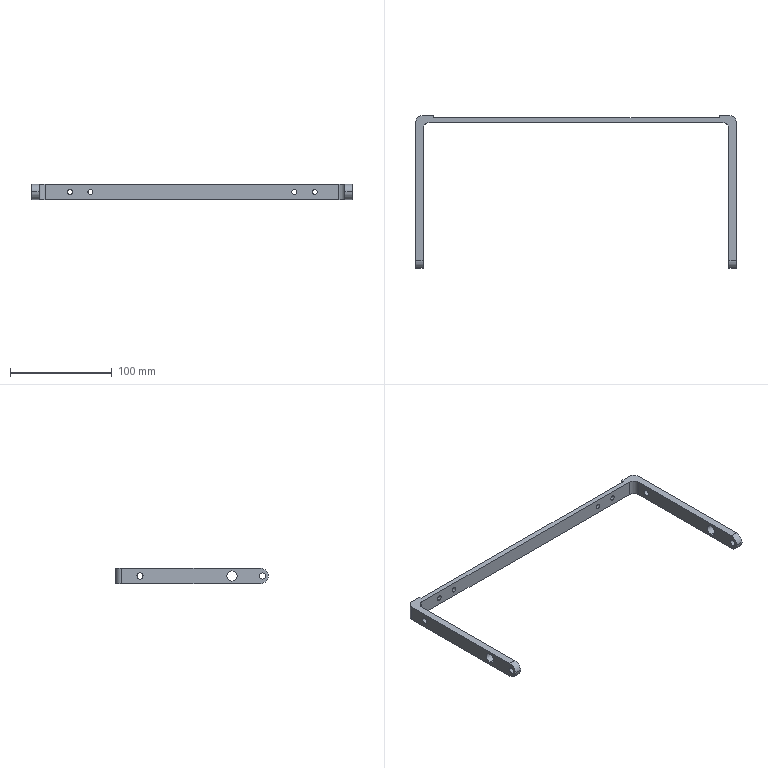Part | SolidWorks | features ICE 3, Fillet 2, Cut 1, Extrusion 1 | 1 solid | 40 faces | box 314 x 149.984 x 15 mm | volume 51932 mm3 | cylinder 28 | plane 12 | commonest cylinder face diameters 5 x8 6 x8 10 x4 12 x4 16 x4
STEP:
#1=CARTESIAN_POINT('',(157.,30.,2.5));
#2=VERTEX_POINT('',#1);
#3=CARTESIAN_POINT('',(157.,30.,12.5));
#4=VERTEX_POINT('',#3);
#5=CARTESIAN_POINT('',(157.,30.,7.5));
#6=DIRECTION('',(-1.,0.,0.));
#7=DIRECTION('',(0.,0.,1.));
#8=AXIS2_PLACEMENT_3D('',#5,#6,#7);
#9=CIRCLE('',#8,5.);
#10=EDGE_CURVE('',#2,#4,#9,.T.);
#11=ORIENTED_EDGE('',*,*,#10,.F.);
#12=CARTESIAN_POINT('',(150.,30.,2.5));
#13=VERTEX_POINT('',#12);
#14=CARTESIAN_POINT('',(157.,30.,2.5));
#15=DIRECTION('',(-1.,0.,0.));
#16=VECTOR('',#15,1000.);
#17=LINE('',#14,#16);
#18=EDGE_CURVE('',#2,#13,#17,.T.);
#19=ORIENTED_EDGE('',*,*,#18,.T.);
#20=CARTESIAN_POINT('',(150.,30.,12.5));
#21=VERTEX_POINT('',#20);
#22=CARTESIAN_POINT('',(150.,30.,7.5));
#23=DIRECTION('',(1.,0.,0.));
#24=DIRECTION('',(0.,1.,0.));
#25=AXIS2_PLACEMENT_3D('',#22,#23,#24);
#26=CIRCLE('',#25,5.);
#27=EDGE_CURVE('',#21,#13,#26,.T.);
#28=ORIENTED_EDGE('',*,*,#27,.F.);
#29=CARTESIAN_POINT('',(157.,30.,12.5));
#30=DIRECTION('',(-1.,0.,0.));
#31=VECTOR('',#30,1000.);
#32=LINE('',#29,#31);
#33=EDGE_CURVE('',#4,#21,#32,.T.);
#34=ORIENTED_EDGE('',*,*,#33,.F.);
#35=EDGE_LOOP('',(#11,#19,#28,#34));
#36=FACE_OUTER_BOUND('',#35,.T.);
#37=CARTESIAN_POINT('',(157.,30.,7.5));
#38=DIRECTION('',(-1.,0.,0.));
#39=DIRECTION('',(0.,0.,1.));
#40=AXIS2_PLACEMENT_3D('',#37,#38,#39);
#41=CYLINDRICAL_SURFACE('',#40,5.);
#42=ADVANCED_FACE('',(#36),#41,.F.);
#43=CARTESIAN_POINT('',(-150.,30.,2.5));
#44=VERTEX_POINT('',#43);
#45=CARTESIAN_POINT('',(-150.,30.,12.5));
#46=VERTEX_POINT('',#45);
#47=CARTESIAN_POINT('',(-150.,30.,7.5));
#48=DIRECTION('',(-1.,0.,0.));
#49=DIRECTION('',(0.,-1.,0.));
#50=AXIS2_PLACEMENT_3D('',#47,#48,#49);
#51=CIRCLE('',#50,5.);
#52=EDGE_CURVE('',#44,#46,#51,.T.);
#53=ORIENTED_EDGE('',*,*,#52,.F.);
#54=CARTESIAN_POINT('',(-157.,30.,2.5));
#55=VERTEX_POINT('',#54);
#56=CARTESIAN_POINT('',(157.,30.,2.5));
#57=DIRECTION('',(-1.,0.,0.));
#58=VECTOR('',#57,1000.);
#59=LINE('',#56,#58);
#60=EDGE_CURVE('',#44,#55,#59,.T.);
#61=ORIENTED_EDGE('',*,*,#60,.T.);
#62=CARTESIAN_POINT('',(-157.,30.,12.5));
#63=VERTEX_POINT('',#62);
#64=CARTESIAN_POINT('',(-157.,30.,7.5));
#65=DIRECTION('',(-1.,0.,0.));
#66=DIRECTION('',(0.,0.,1.));
#67=AXIS2_PLACEMENT_3D('',#64,#65,#66);
#68=CIRCLE('',#67,5.);
#69=EDGE_CURVE('',#55,#63,#68,.T.);
#70=ORIENTED_EDGE('',*,*,#69,.T.);
#71=CARTESIAN_POINT('',(157.,30.,12.5));
#72=DIRECTION('',(-1.,0.,0.));
#73=VECTOR('',#72,1000.);
#74=LINE('',#71,#73);
#75=EDGE_CURVE('',#46,#63,#74,.T.);
#76=ORIENTED_EDGE('',*,*,#75,.F.);
#77=EDGE_LOOP('',(#53,#61,#70,#76));
#78=FACE_OUTER_BOUND('',#77,.T.);
#79=CARTESIAN_POINT('',(157.,30.,7.5));
#80=DIRECTION('',(-1.,0.,0.));
#81=DIRECTION('',(0.,0.,1.));
#82=AXIS2_PLACEMENT_3D('',#79,#80,#81);
#83=CYLINDRICAL_SURFACE('',#82,5.);
#84=ADVANCED_FACE('',(#78),#83,.F.);
#85=CARTESIAN_POINT('',(120.39,137.174,5.));
#86=VERTEX_POINT('',#85);
#87=CARTESIAN_POINT('',(120.39,137.174,10.));
#88=VERTEX_POINT('',#87);
#89=CARTESIAN_POINT('',(120.39,137.174,7.5));
#90=DIRECTION('',(0.,1.,0.));
#91=DIRECTION('',(-1.,0.,0.));
#92=AXIS2_PLACEMENT_3D('',#89,#90,#91);
#93=CIRCLE('',#92,2.5);
#94=EDGE_CURVE('',#86,#88,#93,.T.);
#95=ORIENTED_EDGE('',*,*,#94,.F.);
#96=CARTESIAN_POINT('',(120.39,142.174,5.));
#97=VERTEX_POINT('',#96);
#98=CARTESIAN_POINT('',(120.39,-137.826,5.));
#99=DIRECTION('',(0.,1.,0.));
#100=VECTOR('',#99,1000.);
#101=LINE('',#98,#100);
#102=EDGE_CURVE('',#86,#97,#101,.T.);
#103=ORIENTED_EDGE('',*,*,#102,.T.);
#104=CARTESIAN_POINT('',(120.39,142.174,10.));
#105=VERTEX_POINT('',#104);
#106=CARTESIAN_POINT('',(120.39,142.174,7.5));
#107=DIRECTION('',(0.,1.,0.));
#108=DIRECTION('',(0.,0.,1.));
#109=AXIS2_PLACEMENT_3D('',#106,#107,#108);
#110=CIRCLE('',#109,2.5);
#111=EDGE_CURVE('',#97,#105,#110,.T.);
#112=ORIENTED_EDGE('',*,*,#111,.T.);
#113=CARTESIAN_POINT('',(120.39,-137.826,10.));
#114=DIRECTION('',(0.,1.,0.));
#115=VECTOR('',#114,1000.);
#116=LINE('',#113,#115);
#117=EDGE_CURVE('',#88,#105,#116,.T.);
#118=ORIENTED_EDGE('',*,*,#117,.F.);
#119=EDGE_LOOP('',(#95,#103,#112,#118));
#120=FACE_OUTER_BOUND('',#119,.T.);
#121=CARTESIAN_POINT('',(120.39,-137.826,7.5));
#122=DIRECTION('',(0.,1.,0.));
#123=DIRECTION('',(0.,0.,1.));
#124=AXIS2_PLACEMENT_3D('',#121,#122,#123);
#125=CYLINDRICAL_SURFACE('',#124,2.5);
#126=ADVANCED_FACE('',(#120),#125,.F.);
#127=CARTESIAN_POINT('',(-99.61,137.174,5.));
#128=VERTEX_POINT('',#127);
#129=CARTESIAN_POINT('',(-99.61,137.174,10.));
#130=VERTEX_POINT('',#129);
#131=CARTESIAN_POINT('',(-99.61,137.174,7.5));
#132=DIRECTION('',(0.,1.,0.));
#133=DIRECTION('',(-1.,0.,0.));
#134=AXIS2_PLACEMENT_3D('',#131,#132,#133);
#135=CIRCLE('',#134,2.5);
#136=EDGE_CURVE('',#128,#130,#135,.T.);
#137=ORIENTED_EDGE('',*,*,#136,.F.);
#138=CARTESIAN_POINT('',(-99.61,142.174,5.));
#139=VERTEX_POINT('',#138);
#140=CARTESIAN_POINT('',(-99.61,-137.826,5.));
#141=DIRECTION('',(0.,1.,0.));
#142=VECTOR('',#141,1000.);
#143=LINE('',#140,#142);
#144=EDGE_CURVE('',#128,#139,#143,.T.);
#145=ORIENTED_EDGE('',*,*,#144,.T.);
#146=CARTESIAN_POINT('',(-99.61,142.174,10.));
#147=VERTEX_POINT('',#146);
#148=CARTESIAN_POINT('',(-99.61,142.174,7.5));
#149=DIRECTION('',(0.,1.,0.));
#150=DIRECTION('',(0.,0.,1.));
#151=AXIS2_PLACEMENT_3D('',#148,#149,#150);
#152=CIRCLE('',#151,2.5);
#153=EDGE_CURVE('',#139,#147,#152,.T.);
#154=ORIENTED_EDGE('',*,*,#153,.T.);
#155=CARTESIAN_POINT('',(-99.61,-137.826,10.));
#156=DIRECTION('',(0.,1.,0.));
#157=VECTOR('',#156,1000.);
#158=LINE('',#155,#157);
#159=EDGE_CURVE('',#130,#147,#158,.T.);
#160=ORIENTED_EDGE('',*,*,#159,.F.);
#161=EDGE_LOOP('',(#137,#145,#154,#160));
#162=FACE_OUTER_BOUND('',#161,.T.);
#163=CARTESIAN_POINT('',(-99.61,-137.826,7.5));
#164=DIRECTION('',(0.,1.,0.));
#165=DIRECTION('',(0.,0.,1.));
#166=AXIS2_PLACEMENT_3D('',#163,#164,#165);
#167=CYLINDRICAL_SURFACE('',#166,2.5);
#168=ADVANCED_FACE('',(#162),#167,.F.);
#169=CARTESIAN_POINT('',(-119.61,137.174,5.));
#170=VERTEX_POINT('',#169);
#171=CARTESIAN_POINT('',(-119.61,137.174,10.));
#172=VERTEX_POINT('',#171);
#173=CARTESIAN_POINT('',(-119.61,137.174,7.5));
#174=DIRECTION('',(0.,1.,0.));
#175=DIRECTION('',(-1.,0.,0.));
#176=AXIS2_PLACEMENT_3D('',#173,#174,#175);
#177=CIRCLE('',#176,2.5);
#178=EDGE_CURVE('',#170,#172,#177,.T.);
#179=ORIENTED_EDGE('',*,*,#178,.F.);
#180=CARTESIAN_POINT('',(-119.61,142.174,5.));
#181=VERTEX_POINT('',#180);
#182=CARTESIAN_POINT('',(-119.61,-137.826,5.));
#183=DIRECTION('',(0.,1.,0.));
#184=VECTOR('',#183,1000.);
#185=LINE('',#182,#184);
#186=EDGE_CURVE('',#170,#181,#185,.T.);
#187=ORIENTED_EDGE('',*,*,#186,.T.);
#188=CARTESIAN_POINT('',(-119.61,142.174,10.));
#189=VERTEX_POINT('',#188);
#190=CARTESIAN_POINT('',(-119.61,142.174,7.5));
#191=DIRECTION('',(0.,1.,0.));
#192=DIRECTION('',(0.,0.,1.));
#193=AXIS2_PLACEMENT_3D('',#190,#191,#192);
#194=CIRCLE('',#193,2.5);
#195=EDGE_CURVE('',#181,#189,#194,.T.);
#196=ORIENTED_EDGE('',*,*,#195,.T.);
#197=CARTESIAN_POINT('',(-119.61,-137.826,10.));
#198=DIRECTION('',(0.,1.,0.));
#199=VECTOR('',#198,1000.);
#200=LINE('',#197,#199);
#201=EDGE_CURVE('',#172,#189,#200,.T.);
#202=ORIENTED_EDGE('',*,*,#201,.F.);
#203=EDGE_LOOP('',(#179,#187,#196,#202));
#204=FACE_OUTER_BOUND('',#203,.T.);
#205=CARTESIAN_POINT('',(-119.61,-137.826,7.5));
#206=DIRECTION('',(0.,1.,0.));
#207=DIRECTION('',(0.,0.,1.));
#208=AXIS2_PLACEMENT_3D('',#205,#206,#207);
#209=CYLINDRICAL_SURFACE('',#208,2.5);
#210=ADVANCED_FACE('',(#204),#209,.F.);
#211=CARTESIAN_POINT('',(100.39,137.174,5.));
#212=VERTEX_POINT('',#211);
#213=CARTESIAN_POINT('',(100.39,137.174,10.));
#214=VERTEX_POINT('',#213);
#215=CARTESIAN_POINT('',(100.39,137.174,7.5));
#216=DIRECTION('',(0.,1.,0.));
#217=DIRECTION('',(-1.,0.,0.));
#218=AXIS2_PLACEMENT_3D('',#215,#216,#217);
#219=CIRCLE('',#218,2.5);
#220=EDGE_CURVE('',#212,#214,#219,.T.);
#221=ORIENTED_EDGE('',*,*,#220,.F.);
#222=CARTESIAN_POINT('',(100.39,142.174,5.));
#223=VERTEX_POINT('',#222);
#224=CARTESIAN_POINT('',(100.39,-137.826,5.));
#225=DIRECTION('',(0.,1.,0.));
#226=VECTOR('',#225,1000.);
#227=LINE('',#224,#226);
#228=EDGE_CURVE('',#212,#223,#227,.T.);
#229=ORIENTED_EDGE('',*,*,#228,.T.);
#230=CARTESIAN_POINT('',(100.39,142.174,10.));
#231=VERTEX_POINT('',#230);
#232=CARTESIAN_POINT('',(100.39,142.174,7.5));
#233=DIRECTION('',(0.,1.,0.));
#234=DIRECTION('',(0.,0.,1.));
#235=AXIS2_PLACEMENT_3D('',#232,#233,#234);
#236=CIRCLE('',#235,2.5);
#237=EDGE_CURVE('',#223,#231,#236,.T.);
#238=ORIENTED_EDGE('',*,*,#237,.T.);
#239=CARTESIAN_POINT('',(100.39,-137.826,10.));
#240=DIRECTION('',(0.,1.,0.));
#241=VECTOR('',#240,1000.);
#242=LINE('',#239,#241);
#243=EDGE_CURVE('',#214,#231,#242,.T.);
#244=ORIENTED_EDGE('',*,*,#243,.F.);
#245=EDGE_LOOP('',(#221,#229,#238,#244));
#246=FACE_OUTER_BOUND('',#245,.T.);
#247=CARTESIAN_POINT('',(100.39,-137.826,7.5));
#248=DIRECTION('',(0.,1.,0.));
#249=DIRECTION('',(0.,0.,1.));
#250=AXIS2_PLACEMENT_3D('',#247,#248,#249);
#251=CYLINDRICAL_SURFACE('',#250,2.5);
#252=ADVANCED_FACE('',(#246),#251,.F.);
#253=CARTESIAN_POINT('',(150.,-2.826,7.5));
#254=VERTEX_POINT('',#253);
#255=CARTESIAN_POINT('',(150.,3.174,7.5));
#256=VERTEX_POINT('',#255);
#257=CARTESIAN_POINT('',(150.,0.1739,7.5));
#258=DIRECTION('',(1.,0.,0.));
#259=DIRECTION('',(0.,1.,0.));
#260=AXIS2_PLACEMENT_3D('',#257,#258,#259);
#261=CIRCLE('',#260,3.);
#262=EDGE_CURVE('',#254,#256,#261,.T.);
#263=ORIENTED_EDGE('',*,*,#262,.F.);
#264=CARTESIAN_POINT('',(157.,-2.826,7.5));
#265=VERTEX_POINT('',#264);
#266=CARTESIAN_POINT('',(-449.,-2.826,7.5));
#267=DIRECTION('',(1.,0.,0.));
#268=VECTOR('',#267,1000.);
#269=LINE('',#266,#268);
#270=EDGE_CURVE('',#254,#265,#269,.T.);
#271=ORIENTED_EDGE('',*,*,#270,.T.);
#272=CARTESIAN_POINT('',(157.,3.174,7.5));
#273=VERTEX_POINT('',#272);
#274=CARTESIAN_POINT('',(157.,0.1739,7.5));
#275=DIRECTION('',(1.,0.,0.));
#276=DIRECTION('',(0.,1.,0.));
#277=AXIS2_PLACEMENT_3D('',#274,#275,#276);
#278=CIRCLE('',#277,3.);
#279=EDGE_CURVE('',#265,#273,#278,.T.);
#280=ORIENTED_EDGE('',*,*,#279,.T.);
#281=CARTESIAN_POINT('',(-449.,3.174,7.5));
#282=DIRECTION('',(1.,0.,0.));
#283=VECTOR('',#282,1000.);
#284=LINE('',#281,#283);
#285=EDGE_CURVE('',#256,#273,#284,.T.);
#286=ORIENTED_EDGE('',*,*,#285,.F.);
#287=EDGE_LOOP('',(#263,#271,#280,#286));
#288=FACE_OUTER_BOUND('',#287,.T.);
#289=CARTESIAN_POINT('',(-449.,0.1739,7.5));
#290=DIRECTION('',(1.,0.,0.));
#291=DIRECTION('',(0.,1.,0.));
#292=AXIS2_PLACEMENT_3D('',#289,#290,#291);
#293=CYLINDRICAL_SURFACE('',#292,3.);
#294=ADVANCED_FACE('',(#288),#293,.F.);
#295=CARTESIAN_POINT('',(150.,117.174,7.5));
#296=VERTEX_POINT('',#295);
#297=CARTESIAN_POINT('',(150.,123.174,7.5));
#298=VERTEX_POINT('',#297);
#299=CARTESIAN_POINT('',(150.,120.174,7.5));
#300=DIRECTION('',(1.,0.,0.));
#301=DIRECTION('',(0.,1.,0.));
#302=AXIS2_PLACEMENT_3D('',#299,#300,#301);
#303=CIRCLE('',#302,3.);
#304=EDGE_CURVE('',#296,#298,#303,.T.);
#305=ORIENTED_EDGE('',*,*,#304,.F.);
#306=CARTESIAN_POINT('',(157.,117.174,7.5));
#307=VERTEX_POINT('',#306);
#308=CARTESIAN_POINT('',(-449.,117.174,7.5));
#309=DIRECTION('',(1.,0.,0.));
#310=VECTOR('',#309,1000.);
#311=LINE('',#308,#310);
#312=EDGE_CURVE('',#296,#307,#311,.T.);
#313=ORIENTED_EDGE('',*,*,#312,.T.);
#314=CARTESIAN_POINT('',(157.,123.174,7.5));
#315=VERTEX_POINT('',#314);
#316=CARTESIAN_POINT('',(157.,120.174,7.5));
#317=DIRECTION('',(1.,0.,0.));
#318=DIRECTION('',(0.,1.,0.));
#319=AXIS2_PLACEMENT_3D('',#316,#317,#318);
#320=CIRCLE('',#319,3.);
#321=EDGE_CURVE('',#307,#315,#320,.T.);
#322=ORIENTED_EDGE('',*,*,#321,.T.);
#323=CARTESIAN_POINT('',(-449.,123.174,7.5));
#324=DIRECTION('',(1.,0.,0.));
#325=VECTOR('',#324,1000.);
#326=LINE('',#323,#325);
#327=EDGE_CURVE('',#298,#315,#326,.T.);
#328=ORIENTED_EDGE('',*,*,#327,.F.);
#329=EDGE_LOOP('',(#305,#313,#322,#328));
#330=FACE_OUTER_BOUND('',#329,.T.);
#331=CARTESIAN_POINT('',(-449.,120.174,7.5));
#332=DIRECTION('',(1.,0.,0.));
#333=DIRECTION('',(0.,1.,0.));
#334=AXIS2_PLACEMENT_3D('',#331,#332,#333);
#335=CYLINDRICAL_SURFACE('',#334,3.);
#336=ADVANCED_FACE('',(#330),#335,.F.);
#337=CARTESIAN_POINT('',(-157.,-2.826,7.5));
#338=VERTEX_POINT('',#337);
#339=CARTESIAN_POINT('',(-157.,3.174,7.5));
#340=VERTEX_POINT('',#339);
#341=CARTESIAN_POINT('',(-157.,0.1739,7.5));
#342=DIRECTION('',(1.,0.,0.));
#343=DIRECTION('',(0.,0.,-1.));
#344=AXIS2_PLACEMENT_3D('',#341,#342,#343);
#345=CIRCLE('',#344,3.);
#346=EDGE_CURVE('',#338,#340,#345,.T.);
#347=ORIENTED_EDGE('',*,*,#346,.F.);
#348=CARTESIAN_POINT('',(-150.,-2.826,7.5));
#349=VERTEX_POINT('',#348);
#350=CARTESIAN_POINT('',(-449.,-2.826,7.5));
#351=DIRECTION('',(1.,0.,0.));
#352=VECTOR('',#351,1000.);
#353=LINE('',#350,#352);
#354=EDGE_CURVE('',#338,#349,#353,.T.);
#355=ORIENTED_EDGE('',*,*,#354,.T.);
#356=CARTESIAN_POINT('',(-150.,3.174,7.5));
#357=VERTEX_POINT('',#356);
#358=CARTESIAN_POINT('',(-150.,0.1739,7.5));
#359=DIRECTION('',(-1.,0.,0.));
#360=DIRECTION('',(0.,-1.,0.));
#361=AXIS2_PLACEMENT_3D('',#358,#359,#360);
#362=CIRCLE('',#361,3.);
#363=EDGE_CURVE('',#357,#349,#362,.T.);
#364=ORIENTED_EDGE('',*,*,#363,.F.);
#365=CARTESIAN_POINT('',(-449.,3.174,7.5));
#366=DIRECTION('',(1.,0.,0.));
#367=VECTOR('',#366,1000.);
#368=LINE('',#365,#367);
#369=EDGE_CURVE('',#340,#357,#368,.T.);
#370=ORIENTED_EDGE('',*,*,#369,.F.);
#371=EDGE_LOOP('',(#347,#355,#364,#370));
#372=FACE_OUTER_BOUND('',#371,.T.);
#373=CARTESIAN_POINT('',(-449.,0.1739,7.5));
#374=DIRECTION('',(1.,0.,0.));
#375=DIRECTION('',(0.,1.,0.));
#376=AXIS2_PLACEMENT_3D('',#373,#374,#375);
#377=CYLINDRICAL_SURFACE('',#376,3.);
#378=ADVANCED_FACE('',(#372),#377,.F.);
#379=CARTESIAN_POINT('',(-157.,117.174,7.5));
#380=VERTEX_POINT('',#379);
#381=CARTESIAN_POINT('',(-157.,123.174,7.5));
#382=VERTEX_POINT('',#381);
#383=CARTESIAN_POINT('',(-157.,120.174,7.5));
#384=DIRECTION('',(1.,0.,0.));
#385=DIRECTION('',(0.,0.,-1.));
#386=AXIS2_PLACEMENT_3D('',#383,#384,#385);
#387=CIRCLE('',#386,3.);
#388=EDGE_CURVE('',#380,#382,#387,.T.);
#389=ORIENTED_EDGE('',*,*,#388,.F.);
#390=CARTESIAN_POINT('',(-150.,117.174,7.5));
#391=VERTEX_POINT('',#390);
#392=CARTESIAN_POINT('',(-449.,117.174,7.5));
#393=DIRECTION('',(1.,0.,0.));
#394=VECTOR('',#393,1000.);
#395=LINE('',#392,#394);
#396=EDGE_CURVE('',#380,#391,#395,.T.);
#397=ORIENTED_EDGE('',*,*,#396,.T.);
#398=CARTESIAN_POINT('',(-150.,123.174,7.5));
#399=VERTEX_POINT('',#398);
#400=CARTESIAN_POINT('',(-150.,120.174,7.5));
#401=DIRECTION('',(-1.,0.,0.));
#402=DIRECTION('',(0.,-1.,0.));
#403=AXIS2_PLACEMENT_3D('',#400,#401,#402);
#404=CIRCLE('',#403,3.);
#405=EDGE_CURVE('',#399,#391,#404,.T.);
#406=ORIENTED_EDGE('',*,*,#405,.F.);
#407=CARTESIAN_POINT('',(-449.,123.174,7.5));
#408=DIRECTION('',(1.,0.,0.));
#409=VECTOR('',#408,1000.);
#410=LINE('',#407,#409);
#411=EDGE_CURVE('',#382,#399,#410,.T.);
#412=ORIENTED_EDGE('',*,*,#411,.F.);
#413=EDGE_LOOP('',(#389,#397,#406,#412));
#414=FACE_OUTER_BOUND('',#413,.T.);
#415=CARTESIAN_POINT('',(-449.,120.174,7.5));
#416=DIRECTION('',(1.,0.,0.));
#417=DIRECTION('',(0.,1.,0.));
#418=AXIS2_PLACEMENT_3D('',#415,#416,#417);
#419=CYLINDRICAL_SURFACE('',#418,3.);
#420=ADVANCED_FACE('',(#414),#419,.F.);
#421=CARTESIAN_POINT('',(-139.61,144.174,15.));
#422=VERTEX_POINT('',#421);
#423=CARTESIAN_POINT('',(-151.,144.174,15.));
#424=VERTEX_POINT('',#423);
#425=CARTESIAN_POINT('',(-157.,144.174,15.));
#426=DIRECTION('',(-1.,0.,0.));
#427=VECTOR('',#426,1000.);
#428=LINE('',#425,#427);
#429=EDGE_CURVE('',#422,#424,#428,.T.);
#430=ORIENTED_EDGE('',*,*,#429,.F.);
#431=CARTESIAN_POINT('',(-139.61,144.174,0.));
#432=VERTEX_POINT('',#431);
#433=CARTESIAN_POINT('',(-139.61,144.174,0.));
#434=DIRECTION('',(0.,0.,1.));
#435=VECTOR('',#434,1000.);
#436=LINE('',#433,#435);
#437=EDGE_CURVE('',#432,#422,#436,.T.);
#438=ORIENTED_EDGE('',*,*,#437,.F.);
#439=CARTESIAN_POINT('',(-151.,144.174,0.));
#440=VERTEX_POINT('',#439);
#441=CARTESIAN_POINT('',(-157.,144.174,0.));
#442=DIRECTION('',(-1.,0.,0.));
#443=VECTOR('',#442,1000.);
#444=LINE('',#441,#443);
#445=EDGE_CURVE('',#432,#440,#444,.T.);
#446=ORIENTED_EDGE('',*,*,#445,.T.);
#447=CARTESIAN_POINT('',(-151.,144.174,15.));
#448=DIRECTION('',(0.,0.,1.));
#449=VECTOR('',#448,1000.);
#450=LINE('',#447,#449);
#451=EDGE_CURVE('',#440,#424,#450,.T.);
#452=ORIENTED_EDGE('',*,*,#451,.T.);
#453=EDGE_LOOP('',(#430,#438,#446,#452));
#454=FACE_OUTER_BOUND('',#453,.T.);
#455=CARTESIAN_POINT('',(-157.,144.174,15.));
#456=DIRECTION('',(0.,-1.,0.));
#457=DIRECTION('',(1.,0.,0.));
#458=AXIS2_PLACEMENT_3D('',#455,#456,#457);
#459=PLANE('',#458);
#460=ADVANCED_FACE('',(#454),#459,.F.);
#461=CARTESIAN_POINT('',(-150.,30.,7.5));
#462=DIRECTION('',(-1.,0.,0.));
#463=DIRECTION('',(0.,-1.,0.));
#464=AXIS2_PLACEMENT_3D('',#461,#462,#463);
#465=CIRCLE('',#464,5.);
#466=EDGE_CURVE('',#46,#44,#465,.T.);
#467=ORIENTED_EDGE('',*,*,#466,.T.);
#468=ORIENTED_EDGE('',*,*,#52,.T.);
#469=EDGE_LOOP('',(#467,#468));
#470=FACE_BOUND('',#469,.T.);
#471=ORIENTED_EDGE('',*,*,#363,.T.);
#472=CARTESIAN_POINT('',(-150.,0.1739,7.5));
#473=DIRECTION('',(-1.,0.,0.));
#474=DIRECTION('',(0.,-1.,0.));
#475=AXIS2_PLACEMENT_3D('',#472,#473,#474);
#476=CIRCLE('',#475,3.);
#477=EDGE_CURVE('',#349,#357,#476,.T.);
#478=ORIENTED_EDGE('',*,*,#477,.T.);
#479=EDGE_LOOP('',(#471,#478));
#480=FACE_BOUND('',#479,.T.);
#481=ORIENTED_EDGE('',*,*,#405,.T.);
#482=CARTESIAN_POINT('',(-150.,120.174,7.5));
#483=DIRECTION('',(-1.,0.,0.));
#484=DIRECTION('',(0.,-1.,0.));
#485=AXIS2_PLACEMENT_3D('',#482,#483,#484);
#486=CIRCLE('',#485,3.);
#487=EDGE_CURVE('',#391,#399,#486,.T.);
#488=ORIENTED_EDGE('',*,*,#487,.T.);
#489=EDGE_LOOP('',(#481,#488));
#490=FACE_BOUND('',#489,.T.);
#491=CARTESIAN_POINT('',(-150.,2.174,0.));
#492=VERTEX_POINT('',#491);
#493=CARTESIAN_POINT('',(-150.,131.174,0.));
#494=VERTEX_POINT('',#493);
#495=CARTESIAN_POINT('',(-150.,137.174,0.));
#496=DIRECTION('',(0.,1.,0.));
#497=VECTOR('',#496,1000.);
#498=LINE('',#495,#497);
#499=EDGE_CURVE('',#492,#494,#498,.T.);
#500=ORIENTED_EDGE('',*,*,#499,.T.);
#501=CARTESIAN_POINT('',(-150.,131.174,15.));
#502=VERTEX_POINT('',#501);
#503=CARTESIAN_POINT('',(-150.,131.174,15.));
#504=DIRECTION('',(0.,0.,1.));
#505=VECTOR('',#504,1000.);
#506=LINE('',#503,#505);
#507=EDGE_CURVE('',#494,#502,#506,.T.);
#508=ORIENTED_EDGE('',*,*,#507,.T.);
#509=CARTESIAN_POINT('',(-150.,2.174,15.));
#510=VERTEX_POINT('',#509);
#511=CARTESIAN_POINT('',(-150.,137.174,15.));
#512=DIRECTION('',(0.,1.,0.));
#513=VECTOR('',#512,1000.);
#514=LINE('',#511,#513);
#515=EDGE_CURVE('',#510,#502,#514,.T.);
#516=ORIENTED_EDGE('',*,*,#515,.F.);
#517=CARTESIAN_POINT('',(-150.,-5.81,7.5));
#518=VERTEX_POINT('',#517);
#519=CARTESIAN_POINT('',(-150.,2.174,7.));
#520=DIRECTION('',(1.,0.,0.));
#521=DIRECTION('',(0.,-1.,0.));
#522=AXIS2_PLACEMENT_3D('',#519,#520,#521);
#523=CIRCLE('',#522,8.);
#524=EDGE_CURVE('',#510,#518,#523,.T.);
#525=ORIENTED_EDGE('',*,*,#524,.T.);
#526=CARTESIAN_POINT('',(-150.,2.174,8.));
#527=DIRECTION('',(1.,0.,0.));
#528=DIRECTION('',(0.,-1.,0.));
#529=AXIS2_PLACEMENT_3D('',#526,#527,#528);
#530=CIRCLE('',#529,8.);
#531=EDGE_CURVE('',#518,#492,#530,.T.);
#532=ORIENTED_EDGE('',*,*,#531,.T.);
#533=EDGE_LOOP('',(#500,#508,#516,#525,#532));
#534=FACE_OUTER_BOUND('',#533,.T.);
#535=CARTESIAN_POINT('',(-150.,137.174,15.));
#536=DIRECTION('',(-1.,0.,0.));
#537=DIRECTION('',(0.,-1.,0.));
#538=AXIS2_PLACEMENT_3D('',#535,#536,#537);
#539=PLANE('',#538);
#540=ADVANCED_FACE('',(#470,#480,#490,#534),#539,.F.);
#541=CARTESIAN_POINT('',(120.39,137.174,7.5));
#542=DIRECTION('',(0.,1.,0.));
#543=DIRECTION('',(-1.,0.,0.));
#544=AXIS2_PLACEMENT_3D('',#541,#542,#543);
#545=CIRCLE('',#544,2.5);
#546=EDGE_CURVE('',#88,#86,#545,.T.);
#547=ORIENTED_EDGE('',*,*,#546,.T.);
#548=ORIENTED_EDGE('',*,*,#94,.T.);
#549=EDGE_LOOP('',(#547,#548));
#550=FACE_BOUND('',#549,.T.);
#551=CARTESIAN_POINT('',(-99.61,137.174,7.5));
#552=DIRECTION('',(0.,1.,0.));
#553=DIRECTION('',(-1.,0.,0.));
#554=AXIS2_PLACEMENT_3D('',#551,#552,#553);
#555=CIRCLE('',#554,2.5);
#556=EDGE_CURVE('',#130,#128,#555,.T.);
#557=ORIENTED_EDGE('',*,*,#556,.T.);
#558=ORIENTED_EDGE('',*,*,#136,.T.);
#559=EDGE_LOOP('',(#557,#558));
#560=FACE_BOUND('',#559,.T.);
#561=CARTESIAN_POINT('',(-119.61,137.174,7.5));
#562=DIRECTION('',(0.,1.,0.));
#563=DIRECTION('',(-1.,0.,0.));
#564=AXIS2_PLACEMENT_3D('',#561,#562,#563);
#565=CIRCLE('',#564,2.5);
#566=EDGE_CURVE('',#172,#170,#565,.T.);
#567=ORIENTED_EDGE('',*,*,#566,.T.);
#568=ORIENTED_EDGE('',*,*,#178,.T.);
#569=EDGE_LOOP('',(#567,#568));
#570=FACE_BOUND('',#569,.T.);
#571=CARTESIAN_POINT('',(100.39,137.174,7.5));
#572=DIRECTION('',(0.,1.,0.));
#573=DIRECTION('',(-1.,0.,0.));
#574=AXIS2_PLACEMENT_3D('',#571,#572,#573);
#575=CIRCLE('',#574,2.5);
#576=EDGE_CURVE('',#214,#212,#575,.T.);
#577=ORIENTED_EDGE('',*,*,#576,.T.);
#578=ORIENTED_EDGE('',*,*,#220,.T.);
#579=EDGE_LOOP('',(#577,#578));
#580=FACE_BOUND('',#579,.T.);
#581=CARTESIAN_POINT('',(-144.,137.174,15.));
#582=VERTEX_POINT('',#581);
#583=CARTESIAN_POINT('',(144.,137.174,15.));
#584=VERTEX_POINT('',#583);
#585=CARTESIAN_POINT('',(150.,137.174,15.));
#586=DIRECTION('',(1.,0.,0.));
#587=VECTOR('',#586,1000.);
#588=LINE('',#585,#587);
#589=EDGE_CURVE('',#582,#584,#588,.T.);
#590=ORIENTED_EDGE('',*,*,#589,.F.);
#591=CARTESIAN_POINT('',(-144.,137.174,0.));
#592=VERTEX_POINT('',#591);
#593=CARTESIAN_POINT('',(-144.,137.174,0.));
#594=DIRECTION('',(0.,0.,-1.));
#595=VECTOR('',#594,1000.);
#596=LINE('',#593,#595);
#597=EDGE_CURVE('',#582,#592,#596,.T.);
#598=ORIENTED_EDGE('',*,*,#597,.T.);
#599=CARTESIAN_POINT('',(144.,137.174,0.));
#600=VERTEX_POINT('',#599);
#601=CARTESIAN_POINT('',(150.,137.174,0.));
#602=DIRECTION('',(1.,0.,0.));
#603=VECTOR('',#602,1000.);
#604=LINE('',#601,#603);
#605=EDGE_CURVE('',#592,#600,#604,.T.);
#606=ORIENTED_EDGE('',*,*,#605,.T.);
#607=CARTESIAN_POINT('',(144.,137.174,15.));
#608=DIRECTION('',(0.,0.,1.));
#609=VECTOR('',#608,1000.);
#610=LINE('',#607,#609);
#611=EDGE_CURVE('',#600,#584,#610,.T.);
#612=ORIENTED_EDGE('',*,*,#611,.T.);
#613=EDGE_LOOP('',(#590,#598,#606,#612));
#614=FACE_OUTER_BOUND('',#613,.T.);
#615=CARTESIAN_POINT('',(150.,137.174,15.));
#616=DIRECTION('',(0.,1.,0.));
#617=DIRECTION('',(-1.,0.,0.));
#618=AXIS2_PLACEMENT_3D('',#615,#616,#617);
#619=PLANE('',#618);
#620=ADVANCED_FACE('',(#550,#560,#570,#580,#614),#619,.F.);
#621=ORIENTED_EDGE('',*,*,#27,.T.);
#622=CARTESIAN_POINT('',(150.,30.,7.5));
#623=DIRECTION('',(1.,0.,0.));
#624=DIRECTION('',(0.,1.,0.));
#625=AXIS2_PLACEMENT_3D('',#622,#623,#624);
#626=CIRCLE('',#625,5.);
#627=EDGE_CURVE('',#13,#21,#626,.T.);
#628=ORIENTED_EDGE('',*,*,#627,.T.);
#629=EDGE_LOOP('',(#621,#628));
#630=FACE_BOUND('',#629,.T.);
#631=CARTESIAN_POINT('',(150.,0.1739,7.5));
#632=DIRECTION('',(1.,0.,0.));
#633=DIRECTION('',(0.,1.,0.));
#634=AXIS2_PLACEMENT_3D('',#631,#632,#633);
#635=CIRCLE('',#634,3.);
#636=EDGE_CURVE('',#256,#254,#635,.T.);
#637=ORIENTED_EDGE('',*,*,#636,.T.);
#638=ORIENTED_EDGE('',*,*,#262,.T.);
#639=EDGE_LOOP('',(#637,#638));
#640=FACE_BOUND('',#639,.T.);
#641=CARTESIAN_POINT('',(150.,120.174,7.5));
#642=DIRECTION('',(1.,0.,0.));
#643=DIRECTION('',(0.,1.,0.));
#644=AXIS2_PLACEMENT_3D('',#641,#642,#643);
#645=CIRCLE('',#644,3.);
#646=EDGE_CURVE('',#298,#296,#645,.T.);
#647=ORIENTED_EDGE('',*,*,#646,.T.);
#648=ORIENTED_EDGE('',*,*,#304,.T.);
#649=EDGE_LOOP('',(#647,#648));
#650=FACE_BOUND('',#649,.T.);
#651=CARTESIAN_POINT('',(150.,131.174,15.));
#652=VERTEX_POINT('',#651);
#653=CARTESIAN_POINT('',(150.,2.174,15.));
#654=VERTEX_POINT('',#653);
#655=CARTESIAN_POINT('',(150.,-5.826,15.));
#656=DIRECTION('',(0.,-1.,0.));
#657=VECTOR('',#656,1000.);
#658=LINE('',#655,#657);
#659=EDGE_CURVE('',#652,#654,#658,.T.);
#660=ORIENTED_EDGE('',*,*,#659,.F.);
#661=CARTESIAN_POINT('',(150.,131.174,0.));
#662=VERTEX_POINT('',#661);
#663=CARTESIAN_POINT('',(150.,131.174,0.));
#664=DIRECTION('',(0.,0.,-1.));
#665=VECTOR('',#664,1000.);
#666=LINE('',#663,#665);
#667=EDGE_CURVE('',#652,#662,#666,.T.);
#668=ORIENTED_EDGE('',*,*,#667,.T.);
#669=CARTESIAN_POINT('',(150.,2.174,0.));
#670=VERTEX_POINT('',#669);
#671=CARTESIAN_POINT('',(150.,-5.826,0.));
#672=DIRECTION('',(0.,-1.,0.));
#673=VECTOR('',#672,1000.);
#674=LINE('',#671,#673);
#675=EDGE_CURVE('',#662,#670,#674,.T.);
#676=ORIENTED_EDGE('',*,*,#675,.T.);
#677=CARTESIAN_POINT('',(150.,-5.81,7.5));
#678=VERTEX_POINT('',#677);
#679=CARTESIAN_POINT('',(150.,2.174,8.));
#680=DIRECTION('',(-1.,0.,0.));
#681=DIRECTION('',(0.,1.,0.));
#682=AXIS2_PLACEMENT_3D('',#679,#680,#681);
#683=CIRCLE('',#682,8.);
#684=EDGE_CURVE('',#670,#678,#683,.T.);
#685=ORIENTED_EDGE('',*,*,#684,.T.);
#686=CARTESIAN_POINT('',(150.,2.174,7.));
#687=DIRECTION('',(-1.,0.,0.));
#688=DIRECTION('',(0.,1.,0.));
#689=AXIS2_PLACEMENT_3D('',#686,#687,#688);
#690=CIRCLE('',#689,8.);
#691=EDGE_CURVE('',#678,#654,#690,.T.);
#692=ORIENTED_EDGE('',*,*,#691,.T.);
#693=EDGE_LOOP('',(#660,#668,#676,#685,#692));
#694=FACE_OUTER_BOUND('',#693,.T.);
#695=CARTESIAN_POINT('',(150.,-5.826,15.));
#696=DIRECTION('',(1.,0.,0.));
#697=DIRECTION('',(0.,1.,0.));
#698=AXIS2_PLACEMENT_3D('',#695,#696,#697);
#699=PLANE('',#698);
#700=ADVANCED_FACE('',(#630,#640,#650,#694),#699,.F.);
#701=CARTESIAN_POINT('',(157.,30.,7.5));
#702=DIRECTION('',(-1.,0.,0.));
#703=DIRECTION('',(0.,0.,1.));
#704=AXIS2_PLACEMENT_3D('',#701,#702,#703);
#705=CIRCLE('',#704,5.);
#706=EDGE_CURVE('',#4,#2,#705,.T.);
#707=ORIENTED_EDGE('',*,*,#706,.T.);
#708=ORIENTED_EDGE('',*,*,#10,.T.);
#709=EDGE_LOOP('',(#707,#708));
#710=FACE_BOUND('',#709,.T.);
#711=CARTESIAN_POINT('',(157.,0.1739,7.5));
#712=DIRECTION('',(1.,0.,0.));
#713=DIRECTION('',(0.,1.,0.));
#714=AXIS2_PLACEMENT_3D('',#711,#712,#713);
#715=CIRCLE('',#714,3.);
#716=EDGE_CURVE('',#273,#265,#715,.T.);
#717=ORIENTED_EDGE('',*,*,#716,.F.);
#718=ORIENTED_EDGE('',*,*,#279,.F.);
#719=EDGE_LOOP('',(#717,#718));
#720=FACE_BOUND('',#719,.T.);
#721=CARTESIAN_POINT('',(157.,120.174,7.5));
#722=DIRECTION('',(1.,0.,0.));
#723=DIRECTION('',(0.,1.,0.));
#724=AXIS2_PLACEMENT_3D('',#721,#722,#723);
#725=CIRCLE('',#724,3.);
#726=EDGE_CURVE('',#315,#307,#725,.T.);
#727=ORIENTED_EDGE('',*,*,#726,.F.);
#728=ORIENTED_EDGE('',*,*,#321,.F.);
#729=EDGE_LOOP('',(#727,#728));
#730=FACE_BOUND('',#729,.T.);
#731=CARTESIAN_POINT('',(157.,2.174,0.));
#732=VERTEX_POINT('',#731);
#733=CARTESIAN_POINT('',(157.,138.174,0.));
#734=VERTEX_POINT('',#733);
#735=CARTESIAN_POINT('',(157.,144.174,0.));
#736=DIRECTION('',(0.,1.,0.));
#737=VECTOR('',#736,1000.);
#738=LINE('',#735,#737);
#739=EDGE_CURVE('',#732,#734,#738,.T.);
#740=ORIENTED_EDGE('',*,*,#739,.T.);
#741=CARTESIAN_POINT('',(157.,138.174,15.));
#742=VERTEX_POINT('',#741);
#743=CARTESIAN_POINT('',(157.,138.174,15.));
#744=DIRECTION('',(0.,0.,1.));
#745=VECTOR('',#744,1000.);
#746=LINE('',#743,#745);
#747=EDGE_CURVE('',#734,#742,#746,.T.);
#748=ORIENTED_EDGE('',*,*,#747,.T.);
#749=CARTESIAN_POINT('',(157.,2.174,15.));
#750=VERTEX_POINT('',#749);
#751=CARTESIAN_POINT('',(157.,144.174,15.));
#752=DIRECTION('',(0.,1.,0.));
#753=VECTOR('',#752,1000.);
#754=LINE('',#751,#753);
#755=EDGE_CURVE('',#750,#742,#754,.T.);
#756=ORIENTED_EDGE('',*,*,#755,.F.);
#757=CARTESIAN_POINT('',(157.,-5.81,7.5));
#758=VERTEX_POINT('',#757);
#759=CARTESIAN_POINT('',(157.,2.174,7.));
#760=DIRECTION('',(1.,0.,0.));
#761=DIRECTION('',(0.,-1.,0.));
#762=AXIS2_PLACEMENT_3D('',#759,#760,#761);
#763=CIRCLE('',#762,8.);
#764=EDGE_CURVE('',#750,#758,#763,.T.);
#765=ORIENTED_EDGE('',*,*,#764,.T.);
#766=CARTESIAN_POINT('',(157.,2.174,8.));
#767=DIRECTION('',(1.,0.,0.));
#768=DIRECTION('',(0.,-1.,0.));
#769=AXIS2_PLACEMENT_3D('',#766,#767,#768);
#770=CIRCLE('',#769,8.);
#771=EDGE_CURVE('',#758,#732,#770,.T.);
#772=ORIENTED_EDGE('',*,*,#771,.T.);
#773=EDGE_LOOP('',(#740,#748,#756,#765,#772));
#774=FACE_OUTER_BOUND('',#773,.T.);
#775=CARTESIAN_POINT('',(157.,144.174,15.));
#776=DIRECTION('',(-1.,0.,0.));
#777=DIRECTION('',(0.,-1.,0.));
#778=AXIS2_PLACEMENT_3D('',#775,#776,#777);
#779=PLANE('',#778);
#780=ADVANCED_FACE('',(#710,#720,#730,#774),#779,.F.);
#781=CARTESIAN_POINT('',(151.,144.174,0.));
#782=VERTEX_POINT('',#781);
#783=CARTESIAN_POINT('',(140.39,144.174,0.));
#784=VERTEX_POINT('',#783);
#785=CARTESIAN_POINT('',(-157.,144.174,0.));
#786=DIRECTION('',(-1.,0.,0.));
#787=VECTOR('',#786,1000.);
#788=LINE('',#785,#787);
#789=EDGE_CURVE('',#782,#784,#788,.T.);
#790=ORIENTED_EDGE('',*,*,#789,.T.);
#791=CARTESIAN_POINT('',(140.39,144.174,15.));
#792=VERTEX_POINT('',#791);
#793=CARTESIAN_POINT('',(140.39,144.174,0.));
#794=DIRECTION('',(0.,0.,-1.));
#795=VECTOR('',#794,1000.);
#796=LINE('',#793,#795);
#797=EDGE_CURVE('',#792,#784,#796,.T.);
#798=ORIENTED_EDGE('',*,*,#797,.F.);
#799=CARTESIAN_POINT('',(151.,144.174,15.));
#800=VERTEX_POINT('',#799);
#801=CARTESIAN_POINT('',(-157.,144.174,15.));
#802=DIRECTION('',(-1.,0.,0.));
#803=VECTOR('',#802,1000.);
#804=LINE('',#801,#803);
#805=EDGE_CURVE('',#800,#792,#804,.T.);
#806=ORIENTED_EDGE('',*,*,#805,.F.);
#807=CARTESIAN_POINT('',(151.,144.174,15.));
#808=DIRECTION('',(0.,0.,-1.));
#809=VECTOR('',#808,1000.);
#810=LINE('',#807,#809);
#811=EDGE_CURVE('',#800,#782,#810,.T.);
#812=ORIENTED_EDGE('',*,*,#811,.T.);
#813=EDGE_LOOP('',(#790,#798,#806,#812));
#814=FACE_OUTER_BOUND('',#813,.T.);
#815=CARTESIAN_POINT('',(-157.,144.174,15.));
#816=DIRECTION('',(0.,-1.,0.));
#817=DIRECTION('',(1.,0.,0.));
#818=AXIS2_PLACEMENT_3D('',#815,#816,#817);
#819=PLANE('',#818);
#820=ADVANCED_FACE('',(#814),#819,.F.);
#821=CARTESIAN_POINT('',(-157.,30.,7.5));
#822=DIRECTION('',(-1.,0.,0.));
#823=DIRECTION('',(0.,0.,1.));
#824=AXIS2_PLACEMENT_3D('',#821,#822,#823);
#825=CIRCLE('',#824,5.);
#826=EDGE_CURVE('',#63,#55,#825,.T.);
#827=ORIENTED_EDGE('',*,*,#826,.F.);
#828=ORIENTED_EDGE('',*,*,#69,.F.);
#829=EDGE_LOOP('',(#827,#828));
#830=FACE_BOUND('',#829,.T.);
#831=CARTESIAN_POINT('',(-157.,0.1739,7.5));
#832=DIRECTION('',(1.,0.,0.));
#833=DIRECTION('',(0.,0.,-1.));
#834=AXIS2_PLACEMENT_3D('',#831,#832,#833);
#835=CIRCLE('',#834,3.);
#836=EDGE_CURVE('',#340,#338,#835,.T.);
#837=ORIENTED_EDGE('',*,*,#836,.T.);
#838=ORIENTED_EDGE('',*,*,#346,.T.);
#839=EDGE_LOOP('',(#837,#838));
#840=FACE_BOUND('',#839,.T.);
#841=CARTESIAN_POINT('',(-157.,120.174,7.5));
#842=DIRECTION('',(1.,0.,0.));
#843=DIRECTION('',(0.,0.,-1.));
#844=AXIS2_PLACEMENT_3D('',#841,#842,#843);
#845=CIRCLE('',#844,3.);
#846=EDGE_CURVE('',#382,#380,#845,.T.);
#847=ORIENTED_EDGE('',*,*,#846,.T.);
#848=ORIENTED_EDGE('',*,*,#388,.T.);
#849=EDGE_LOOP('',(#847,#848));
#850=FACE_BOUND('',#849,.T.);
#851=CARTESIAN_POINT('',(-157.,138.174,15.));
#852=VERTEX_POINT('',#851);
#853=CARTESIAN_POINT('',(-157.,2.174,15.));
#854=VERTEX_POINT('',#853);
#855=CARTESIAN_POINT('',(-157.,-5.826,15.));
#856=DIRECTION('',(0.,-1.,0.));
#857=VECTOR('',#856,1000.);
#858=LINE('',#855,#857);
#859=EDGE_CURVE('',#852,#854,#858,.T.);
#860=ORIENTED_EDGE('',*,*,#859,.F.);
#861=CARTESIAN_POINT('',(-157.,138.174,0.));
#862=VERTEX_POINT('',#861);
#863=CARTESIAN_POINT('',(-157.,138.174,15.));
#864=DIRECTION('',(0.,0.,-1.));
#865=VECTOR('',#864,1000.);
#866=LINE('',#863,#865);
#867=EDGE_CURVE('',#852,#862,#866,.T.);
#868=ORIENTED_EDGE('',*,*,#867,.T.);
#869=CARTESIAN_POINT('',(-157.,2.174,0.));
#870=VERTEX_POINT('',#869);
#871=CARTESIAN_POINT('',(-157.,-5.826,0.));
#872=DIRECTION('',(0.,-1.,0.));
#873=VECTOR('',#872,1000.);
#874=LINE('',#871,#873);
#875=EDGE_CURVE('',#862,#870,#874,.T.);
#876=ORIENTED_EDGE('',*,*,#875,.T.);
#877=CARTESIAN_POINT('',(-157.,-5.81,7.5));
#878=VERTEX_POINT('',#877);
#879=CARTESIAN_POINT('',(-157.,2.174,8.));
#880=DIRECTION('',(-1.,0.,0.));
#881=DIRECTION('',(0.,0.,-1.));
#882=AXIS2_PLACEMENT_3D('',#879,#880,#881);
#883=CIRCLE('',#882,8.);
#884=EDGE_CURVE('',#870,#878,#883,.T.);
#885=ORIENTED_EDGE('',*,*,#884,.T.);
#886=CARTESIAN_POINT('',(-157.,2.174,7.));
#887=DIRECTION('',(-1.,0.,0.));
#888=DIRECTION('',(0.,0.,-1.));
#889=AXIS2_PLACEMENT_3D('',#886,#887,#888);
#890=CIRCLE('',#889,8.);
#891=EDGE_CURVE('',#878,#854,#890,.T.);
#892=ORIENTED_EDGE('',*,*,#891,.T.);
#893=EDGE_LOOP('',(#860,#868,#876,#885,#892));
#894=FACE_OUTER_BOUND('',#893,.T.);
#895=CARTESIAN_POINT('',(-157.,-5.826,15.));
#896=DIRECTION('',(1.,0.,0.));
#897=DIRECTION('',(0.,0.,-1.));
#898=AXIS2_PLACEMENT_3D('',#895,#896,#897);
#899=PLANE('',#898);
#900=ADVANCED_FACE('',(#830,#840,#850,#894),#899,.F.);
#901=CARTESIAN_POINT('',(-139.61,142.174,15.));
#902=VERTEX_POINT('',#901);
#903=CARTESIAN_POINT('',(140.39,142.174,15.));
#904=VERTEX_POINT('',#903);
#905=CARTESIAN_POINT('',(140.39,142.174,15.));
#906=DIRECTION('',(1.,0.,0.));
#907=VECTOR('',#906,1000.);
#908=LINE('',#905,#907);
#909=EDGE_CURVE('',#902,#904,#908,.T.);
#910=ORIENTED_EDGE('',*,*,#909,.F.);
#911=CARTESIAN_POINT('',(-139.61,142.174,15.));
#912=DIRECTION('',(0.,1.,0.));
#913=VECTOR('',#912,1000.);
#914=LINE('',#911,#913);
#915=EDGE_CURVE('',#902,#422,#914,.T.);
#916=ORIENTED_EDGE('',*,*,#915,.T.);
#917=ORIENTED_EDGE('',*,*,#429,.T.);
#918=CARTESIAN_POINT('',(-151.,138.174,15.));
#919=DIRECTION('',(0.,0.,1.));
#920=DIRECTION('',(-1.,0.,0.));
#921=AXIS2_PLACEMENT_3D('',#918,#919,#920);
#922=CIRCLE('',#921,6.);
#923=EDGE_CURVE('',#424,#852,#922,.T.);
#924=ORIENTED_EDGE('',*,*,#923,.T.);
#925=ORIENTED_EDGE('',*,*,#859,.T.);
#926=CARTESIAN_POINT('',(0.,2.174,15.));
#927=DIRECTION('',(1.,0.,0.));
#928=VECTOR('',#927,1000.);
#929=LINE('',#926,#928);
#930=EDGE_CURVE('',#854,#510,#929,.T.);
#931=ORIENTED_EDGE('',*,*,#930,.T.);
#932=ORIENTED_EDGE('',*,*,#515,.T.);
#933=CARTESIAN_POINT('',(-144.,131.174,15.));
#934=DIRECTION('',(0.,0.,-1.));
#935=DIRECTION('',(-1.,0.,0.));
#936=AXIS2_PLACEMENT_3D('',#933,#934,#935);
#937=CIRCLE('',#936,6.);
#938=EDGE_CURVE('',#502,#582,#937,.T.);
#939=ORIENTED_EDGE('',*,*,#938,.T.);
#940=ORIENTED_EDGE('',*,*,#589,.T.);
#941=CARTESIAN_POINT('',(144.,131.174,15.));
#942=DIRECTION('',(0.,0.,-1.));
#943=DIRECTION('',(-1.,0.,0.));
#944=AXIS2_PLACEMENT_3D('',#941,#942,#943);
#945=CIRCLE('',#944,6.);
#946=EDGE_CURVE('',#584,#652,#945,.T.);
#947=ORIENTED_EDGE('',*,*,#946,.T.);
#948=ORIENTED_EDGE('',*,*,#659,.T.);
#949=CARTESIAN_POINT('',(0.,2.174,15.));
#950=DIRECTION('',(1.,0.,0.));
#951=VECTOR('',#950,1000.);
#952=LINE('',#949,#951);
#953=EDGE_CURVE('',#654,#750,#952,.T.);
#954=ORIENTED_EDGE('',*,*,#953,.T.);
#955=ORIENTED_EDGE('',*,*,#755,.T.);
#956=CARTESIAN_POINT('',(151.,138.174,15.));
#957=DIRECTION('',(0.,0.,1.));
#958=DIRECTION('',(-1.,0.,0.));
#959=AXIS2_PLACEMENT_3D('',#956,#957,#958);
#960=CIRCLE('',#959,6.);
#961=EDGE_CURVE('',#742,#800,#960,.T.);
#962=ORIENTED_EDGE('',*,*,#961,.T.);
#963=ORIENTED_EDGE('',*,*,#805,.T.);
#964=CARTESIAN_POINT('',(140.39,142.174,15.));
#965=DIRECTION('',(0.,1.,0.));
#966=VECTOR('',#965,1000.);
#967=LINE('',#964,#966);
#968=EDGE_CURVE('',#904,#792,#967,.T.);
#969=ORIENTED_EDGE('',*,*,#968,.F.);
#970=EDGE_LOOP('',(#910,#916,#917,#924,#925,#931,#932,#939,#940,#947,#948,#954,#955,#962,#963,#969));
#971=FACE_OUTER_BOUND('',#970,.T.);
#972=CARTESIAN_POINT('',(0.,0.,15.));
#973=DIRECTION('',(0.,0.,-1.));
#974=DIRECTION('',(-1.,0.,0.));
#975=AXIS2_PLACEMENT_3D('',#972,#973,#974);
#976=PLANE('',#975);
#977=ADVANCED_FACE('',(#971),#976,.F.);
#978=CARTESIAN_POINT('',(-139.61,142.174,0.));
#979=VERTEX_POINT('',#978);
#980=CARTESIAN_POINT('',(-139.61,142.174,0.));
#981=DIRECTION('',(0.,1.,0.));
#982=VECTOR('',#981,1000.);
#983=LINE('',#980,#982);
#984=EDGE_CURVE('',#979,#432,#983,.T.);
#985=ORIENTED_EDGE('',*,*,#984,.F.);
#986=CARTESIAN_POINT('',(140.39,142.174,0.));
#987=VERTEX_POINT('',#986);
#988=CARTESIAN_POINT('',(140.39,142.174,0.));
#989=DIRECTION('',(-1.,0.,0.));
#990=VECTOR('',#989,1000.);
#991=LINE('',#988,#990);
#992=EDGE_CURVE('',#987,#979,#991,.T.);
#993=ORIENTED_EDGE('',*,*,#992,.F.);
#994=CARTESIAN_POINT('',(140.39,142.174,0.));
#995=DIRECTION('',(0.,1.,0.));
#996=VECTOR('',#995,1000.);
#997=LINE('',#994,#996);
#998=EDGE_CURVE('',#987,#784,#997,.T.);
#999=ORIENTED_EDGE('',*,*,#998,.T.);
#1000=ORIENTED_EDGE('',*,*,#789,.F.);
#1001=CARTESIAN_POINT('',(151.,138.174,0.));
#1002=DIRECTION('',(0.,0.,-1.));
#1003=DIRECTION('',(-1.,0.,0.));
#1004=AXIS2_PLACEMENT_3D('',#1001,#1002,#1003);
#1005=CIRCLE('',#1004,6.);
#1006=EDGE_CURVE('',#782,#734,#1005,.T.);
#1007=ORIENTED_EDGE('',*,*,#1006,.T.);
#1008=ORIENTED_EDGE('',*,*,#739,.F.);
#1009=CARTESIAN_POINT('',(150.,2.174,0.));
#1010=DIRECTION('',(-1.,0.,0.));
#1011=VECTOR('',#1010,1000.);
#1012=LINE('',#1009,#1011);
#1013=EDGE_CURVE('',#732,#670,#1012,.T.);
#1014=ORIENTED_EDGE('',*,*,#1013,.T.);
#1015=ORIENTED_EDGE('',*,*,#675,.F.);
#1016=CARTESIAN_POINT('',(144.,131.174,0.));
#1017=DIRECTION('',(0.,0.,1.));
#1018=DIRECTION('',(-1.,0.,0.));
#1019=AXIS2_PLACEMENT_3D('',#1016,#1017,#1018);
#1020=CIRCLE('',#1019,6.);
#1021=EDGE_CURVE('',#662,#600,#1020,.T.);
#1022=ORIENTED_EDGE('',*,*,#1021,.T.);
#1023=ORIENTED_EDGE('',*,*,#605,.F.);
#1024=CARTESIAN_POINT('',(-144.,131.174,0.));
#1025=DIRECTION('',(0.,0.,1.));
#1026=DIRECTION('',(-1.,0.,0.));
#1027=AXIS2_PLACEMENT_3D('',#1024,#1025,#1026);
#1028=CIRCLE('',#1027,6.);
#1029=EDGE_CURVE('',#592,#494,#1028,.T.);
#1030=ORIENTED_EDGE('',*,*,#1029,.T.);
#1031=ORIENTED_EDGE('',*,*,#499,.F.);
#1032=CARTESIAN_POINT('',(-157.,2.174,0.));
#1033=DIRECTION('',(-1.,0.,0.));
#1034=VECTOR('',#1033,1000.);
#1035=LINE('',#1032,#1034);
#1036=EDGE_CURVE('',#492,#870,#1035,.T.);
#1037=ORIENTED_EDGE('',*,*,#1036,.T.);
#1038=ORIENTED_EDGE('',*,*,#875,.F.);
#1039=CARTESIAN_POINT('',(-151.,138.174,0.));
#1040=DIRECTION('',(0.,0.,-1.));
#1041=DIRECTION('',(-1.,0.,0.));
#1042=AXIS2_PLACEMENT_3D('',#1039,#1040,#1041);
#1043=CIRCLE('',#1042,6.);
#1044=EDGE_CURVE('',#862,#440,#1043,.T.);
#1045=ORIENTED_EDGE('',*,*,#1044,.T.);
#1046=ORIENTED_EDGE('',*,*,#445,.F.);
#1047=EDGE_LOOP('',(#985,#993,#999,#1000,#1007,#1008,#1014,#1015,#1022,#1023,#1030,#1031,#1037,#1038,#1045,#1046));
#1048=FACE_OUTER_BOUND('',#1047,.T.);
#1049=CARTESIAN_POINT('',(0.,0.,0.));
#1050=DIRECTION('',(0.,0.,-1.));
#1051=DIRECTION('',(-1.,0.,0.));
#1052=AXIS2_PLACEMENT_3D('',#1049,#1050,#1051);
#1053=PLANE('',#1052);
#1054=ADVANCED_FACE('',(#1048),#1053,.T.);
#1055=ORIENTED_EDGE('',*,*,#396,.F.);
#1056=ORIENTED_EDGE('',*,*,#846,.F.);
#1057=ORIENTED_EDGE('',*,*,#411,.T.);
#1058=ORIENTED_EDGE('',*,*,#487,.F.);
#1059=EDGE_LOOP('',(#1055,#1056,#1057,#1058));
#1060=FACE_OUTER_BOUND('',#1059,.T.);
#1061=CARTESIAN_POINT('',(-449.,120.174,7.5));
#1062=DIRECTION('',(1.,0.,0.));
#1063=DIRECTION('',(0.,1.,0.));
#1064=AXIS2_PLACEMENT_3D('',#1061,#1062,#1063);
#1065=CYLINDRICAL_SURFACE('',#1064,3.);
#1066=ADVANCED_FACE('',(#1060),#1065,.F.);
#1067=ORIENTED_EDGE('',*,*,#354,.F.);
#1068=ORIENTED_EDGE('',*,*,#836,.F.);
#1069=ORIENTED_EDGE('',*,*,#369,.T.);
#1070=ORIENTED_EDGE('',*,*,#477,.F.);
#1071=EDGE_LOOP('',(#1067,#1068,#1069,#1070));
#1072=FACE_OUTER_BOUND('',#1071,.T.);
#1073=CARTESIAN_POINT('',(-449.,0.1739,7.5));
#1074=DIRECTION('',(1.,0.,0.));
#1075=DIRECTION('',(0.,1.,0.));
#1076=AXIS2_PLACEMENT_3D('',#1073,#1074,#1075);
#1077=CYLINDRICAL_SURFACE('',#1076,3.);
#1078=ADVANCED_FACE('',(#1072),#1077,.F.);
#1079=ORIENTED_EDGE('',*,*,#312,.F.);
#1080=ORIENTED_EDGE('',*,*,#646,.F.);
#1081=ORIENTED_EDGE('',*,*,#327,.T.);
#1082=ORIENTED_EDGE('',*,*,#726,.T.);
#1083=EDGE_LOOP('',(#1079,#1080,#1081,#1082));
#1084=FACE_OUTER_BOUND('',#1083,.T.);
#1085=CARTESIAN_POINT('',(-449.,120.174,7.5));
#1086=DIRECTION('',(1.,0.,0.));
#1087=DIRECTION('',(0.,1.,0.));
#1088=AXIS2_PLACEMENT_3D('',#1085,#1086,#1087);
#1089=CYLINDRICAL_SURFACE('',#1088,3.);
#1090=ADVANCED_FACE('',(#1084),#1089,.F.);
#1091=ORIENTED_EDGE('',*,*,#270,.F.);
#1092=ORIENTED_EDGE('',*,*,#636,.F.);
#1093=ORIENTED_EDGE('',*,*,#285,.T.);
#1094=ORIENTED_EDGE('',*,*,#716,.T.);
#1095=EDGE_LOOP('',(#1091,#1092,#1093,#1094));
#1096=FACE_OUTER_BOUND('',#1095,.T.);
#1097=CARTESIAN_POINT('',(-449.,0.1739,7.5));
#1098=DIRECTION('',(1.,0.,0.));
#1099=DIRECTION('',(0.,1.,0.));
#1100=AXIS2_PLACEMENT_3D('',#1097,#1098,#1099);
#1101=CYLINDRICAL_SURFACE('',#1100,3.);
#1102=ADVANCED_FACE('',(#1096),#1101,.F.);
#1103=CARTESIAN_POINT('',(-153.5,-5.81,7.5));
#1104=DIRECTION('',(1.,0.,0.));
#1105=VECTOR('',#1104,1000.);
#1106=LINE('',#1103,#1105);
#1107=EDGE_CURVE('',#878,#518,#1106,.T.);
#1108=ORIENTED_EDGE('',*,*,#1107,.F.);
#1109=ORIENTED_EDGE('',*,*,#884,.F.);
#1110=ORIENTED_EDGE('',*,*,#1036,.F.);
#1111=ORIENTED_EDGE('',*,*,#531,.F.);
#1112=EDGE_LOOP('',(#1108,#1109,#1110,#1111));
#1113=FACE_OUTER_BOUND('',#1112,.T.);
#1114=CARTESIAN_POINT('',(-150.,2.174,8.));
#1115=DIRECTION('',(-1.,0.,0.));
#1116=DIRECTION('',(0.,-1.,0.));
#1117=AXIS2_PLACEMENT_3D('',#1114,#1115,#1116);
#1118=CYLINDRICAL_SURFACE('',#1117,8.);
#1119=ADVANCED_FACE('',(#1113),#1118,.T.);
#1120=ORIENTED_EDGE('',*,*,#891,.F.);
#1121=ORIENTED_EDGE('',*,*,#1107,.T.);
#1122=ORIENTED_EDGE('',*,*,#524,.F.);
#1123=ORIENTED_EDGE('',*,*,#930,.F.);
#1124=EDGE_LOOP('',(#1120,#1121,#1122,#1123));
#1125=FACE_OUTER_BOUND('',#1124,.T.);
#1126=CARTESIAN_POINT('',(0.,2.174,7.));
#1127=DIRECTION('',(1.,0.,0.));
#1128=DIRECTION('',(0.,1.,0.));
#1129=AXIS2_PLACEMENT_3D('',#1126,#1127,#1128);
#1130=CYLINDRICAL_SURFACE('',#1129,8.);
#1131=ADVANCED_FACE('',(#1125),#1130,.T.);
#1132=CARTESIAN_POINT('',(153.5,-5.81,7.5));
#1133=DIRECTION('',(1.,0.,0.));
#1134=VECTOR('',#1133,1000.);
#1135=LINE('',#1132,#1134);
#1136=EDGE_CURVE('',#678,#758,#1135,.T.);
#1137=ORIENTED_EDGE('',*,*,#1136,.F.);
#1138=ORIENTED_EDGE('',*,*,#684,.F.);
#1139=ORIENTED_EDGE('',*,*,#1013,.F.);
#1140=ORIENTED_EDGE('',*,*,#771,.F.);
#1141=EDGE_LOOP('',(#1137,#1138,#1139,#1140));
#1142=FACE_OUTER_BOUND('',#1141,.T.);
#1143=CARTESIAN_POINT('',(157.,2.174,8.));
#1144=DIRECTION('',(-1.,0.,0.));
#1145=DIRECTION('',(0.,-1.,0.));
#1146=AXIS2_PLACEMENT_3D('',#1143,#1144,#1145);
#1147=CYLINDRICAL_SURFACE('',#1146,8.);
#1148=ADVANCED_FACE('',(#1142),#1147,.T.);
#1149=ORIENTED_EDGE('',*,*,#691,.F.);
#1150=ORIENTED_EDGE('',*,*,#1136,.T.);
#1151=ORIENTED_EDGE('',*,*,#764,.F.);
#1152=ORIENTED_EDGE('',*,*,#953,.F.);
#1153=EDGE_LOOP('',(#1149,#1150,#1151,#1152));
#1154=FACE_OUTER_BOUND('',#1153,.T.);
#1155=CARTESIAN_POINT('',(0.,2.174,7.));
#1156=DIRECTION('',(1.,0.,0.));
#1157=DIRECTION('',(0.,1.,0.));
#1158=AXIS2_PLACEMENT_3D('',#1155,#1156,#1157);
#1159=CYLINDRICAL_SURFACE('',#1158,8.);
#1160=ADVANCED_FACE('',(#1154),#1159,.T.);
#1161=ORIENTED_EDGE('',*,*,#938,.F.);
#1162=ORIENTED_EDGE('',*,*,#507,.F.);
#1163=ORIENTED_EDGE('',*,*,#1029,.F.);
#1164=ORIENTED_EDGE('',*,*,#597,.F.);
#1165=EDGE_LOOP('',(#1161,#1162,#1163,#1164));
#1166=FACE_OUTER_BOUND('',#1165,.T.);
#1167=CARTESIAN_POINT('',(-144.,131.174,15.));
#1168=DIRECTION('',(0.,0.,1.));
#1169=DIRECTION('',(1.,0.,0.));
#1170=AXIS2_PLACEMENT_3D('',#1167,#1168,#1169);
#1171=CYLINDRICAL_SURFACE('',#1170,6.);
#1172=ADVANCED_FACE('',(#1166),#1171,.F.);
#1173=ORIENTED_EDGE('',*,*,#946,.F.);
#1174=ORIENTED_EDGE('',*,*,#611,.F.);
#1175=ORIENTED_EDGE('',*,*,#1021,.F.);
#1176=ORIENTED_EDGE('',*,*,#667,.F.);
#1177=EDGE_LOOP('',(#1173,#1174,#1175,#1176));
#1178=FACE_OUTER_BOUND('',#1177,.T.);
#1179=CARTESIAN_POINT('',(144.,131.174,15.));
#1180=DIRECTION('',(0.,0.,1.));
#1181=DIRECTION('',(1.,0.,0.));
#1182=AXIS2_PLACEMENT_3D('',#1179,#1180,#1181);
#1183=CYLINDRICAL_SURFACE('',#1182,6.);
#1184=ADVANCED_FACE('',(#1178),#1183,.F.);
#1185=ORIENTED_EDGE('',*,*,#961,.F.);
#1186=ORIENTED_EDGE('',*,*,#747,.F.);
#1187=ORIENTED_EDGE('',*,*,#1006,.F.);
#1188=ORIENTED_EDGE('',*,*,#811,.F.);
#1189=EDGE_LOOP('',(#1185,#1186,#1187,#1188));
#1190=FACE_OUTER_BOUND('',#1189,.T.);
#1191=CARTESIAN_POINT('',(151.,138.174,15.));
#1192=DIRECTION('',(0.,0.,-1.));
#1193=DIRECTION('',(-1.,0.,0.));
#1194=AXIS2_PLACEMENT_3D('',#1191,#1192,#1193);
#1195=CYLINDRICAL_SURFACE('',#1194,6.);
#1196=ADVANCED_FACE('',(#1190),#1195,.T.);
#1197=ORIENTED_EDGE('',*,*,#923,.F.);
#1198=ORIENTED_EDGE('',*,*,#451,.F.);
#1199=ORIENTED_EDGE('',*,*,#1044,.F.);
#1200=ORIENTED_EDGE('',*,*,#867,.F.);
#1201=EDGE_LOOP('',(#1197,#1198,#1199,#1200));
#1202=FACE_OUTER_BOUND('',#1201,.T.);
#1203=CARTESIAN_POINT('',(-151.,138.174,15.));
#1204=DIRECTION('',(0.,0.,-1.));
#1205=DIRECTION('',(-1.,0.,0.));
#1206=AXIS2_PLACEMENT_3D('',#1203,#1204,#1205);
#1207=CYLINDRICAL_SURFACE('',#1206,6.);
#1208=ADVANCED_FACE('',(#1202),#1207,.T.);
#1209=ORIENTED_EDGE('',*,*,#437,.T.);
#1210=ORIENTED_EDGE('',*,*,#915,.F.);
#1211=CARTESIAN_POINT('',(-139.61,142.174,0.));
#1212=DIRECTION('',(0.,0.,1.));
#1213=VECTOR('',#1212,1000.);
#1214=LINE('',#1211,#1213);
#1215=EDGE_CURVE('',#979,#902,#1214,.T.);
#1216=ORIENTED_EDGE('',*,*,#1215,.F.);
#1217=ORIENTED_EDGE('',*,*,#984,.T.);
#1218=EDGE_LOOP('',(#1209,#1210,#1216,#1217));
#1219=FACE_OUTER_BOUND('',#1218,.T.);
#1220=CARTESIAN_POINT('',(-139.61,142.174,0.));
#1221=DIRECTION('',(-1.,0.,0.));
#1222=DIRECTION('',(0.,-1.,0.));
#1223=AXIS2_PLACEMENT_3D('',#1220,#1221,#1222);
#1224=PLANE('',#1223);
#1225=ADVANCED_FACE('',(#1219),#1224,.F.);
#1226=ORIENTED_EDGE('',*,*,#797,.T.);
#1227=ORIENTED_EDGE('',*,*,#998,.F.);
#1228=CARTESIAN_POINT('',(140.39,142.174,0.));
#1229=DIRECTION('',(0.,0.,-1.));
#1230=VECTOR('',#1229,1000.);
#1231=LINE('',#1228,#1230);
#1232=EDGE_CURVE('',#904,#987,#1231,.T.);
#1233=ORIENTED_EDGE('',*,*,#1232,.F.);
#1234=ORIENTED_EDGE('',*,*,#968,.T.);
#1235=EDGE_LOOP('',(#1226,#1227,#1233,#1234));
#1236=FACE_OUTER_BOUND('',#1235,.T.);
#1237=CARTESIAN_POINT('',(140.39,142.174,0.));
#1238=DIRECTION('',(1.,0.,0.));
#1239=DIRECTION('',(0.,1.,0.));
#1240=AXIS2_PLACEMENT_3D('',#1237,#1238,#1239);
#1241=PLANE('',#1240);
#1242=ADVANCED_FACE('',(#1236),#1241,.F.);
#1243=CARTESIAN_POINT('',(120.39,142.174,7.5));
#1244=DIRECTION('',(0.,1.,0.));
#1245=DIRECTION('',(0.,0.,1.));
#1246=AXIS2_PLACEMENT_3D('',#1243,#1244,#1245);
#1247=CIRCLE('',#1246,2.5);
#1248=EDGE_CURVE('',#105,#97,#1247,.T.);
#1249=ORIENTED_EDGE('',*,*,#1248,.F.);
#1250=ORIENTED_EDGE('',*,*,#111,.F.);
#1251=EDGE_LOOP('',(#1249,#1250));
#1252=FACE_BOUND('',#1251,.T.);
#1253=CARTESIAN_POINT('',(-99.61,142.174,7.5));
#1254=DIRECTION('',(0.,1.,0.));
#1255=DIRECTION('',(0.,0.,1.));
#1256=AXIS2_PLACEMENT_3D('',#1253,#1254,#1255);
#1257=CIRCLE('',#1256,2.5);
#1258=EDGE_CURVE('',#147,#139,#1257,.T.);
#1259=ORIENTED_EDGE('',*,*,#1258,.F.);
#1260=ORIENTED_EDGE('',*,*,#153,.F.);
#1261=EDGE_LOOP('',(#1259,#1260));
#1262=FACE_BOUND('',#1261,.T.);
#1263=CARTESIAN_POINT('',(-119.61,142.174,7.5));
#1264=DIRECTION('',(0.,1.,0.));
#1265=DIRECTION('',(0.,0.,1.));
#1266=AXIS2_PLACEMENT_3D('',#1263,#1264,#1265);
#1267=CIRCLE('',#1266,2.5);
#1268=EDGE_CURVE('',#189,#181,#1267,.T.);
#1269=ORIENTED_EDGE('',*,*,#1268,.F.);
#1270=ORIENTED_EDGE('',*,*,#195,.F.);
#1271=EDGE_LOOP('',(#1269,#1270));
#1272=FACE_BOUND('',#1271,.T.);
#1273=CARTESIAN_POINT('',(100.39,142.174,7.5));
#1274=DIRECTION('',(0.,1.,0.));
#1275=DIRECTION('',(0.,0.,1.));
#1276=AXIS2_PLACEMENT_3D('',#1273,#1274,#1275);
#1277=CIRCLE('',#1276,2.5);
#1278=EDGE_CURVE('',#231,#223,#1277,.T.);
#1279=ORIENTED_EDGE('',*,*,#1278,.F.);
#1280=ORIENTED_EDGE('',*,*,#237,.F.);
#1281=EDGE_LOOP('',(#1279,#1280));
#1282=FACE_BOUND('',#1281,.T.);
#1283=ORIENTED_EDGE('',*,*,#1215,.T.);
#1284=ORIENTED_EDGE('',*,*,#909,.T.);
#1285=ORIENTED_EDGE('',*,*,#1232,.T.);
#1286=ORIENTED_EDGE('',*,*,#992,.T.);
#1287=EDGE_LOOP('',(#1283,#1284,#1285,#1286));
#1288=FACE_OUTER_BOUND('',#1287,.T.);
#1289=CARTESIAN_POINT('',(0.,142.174,0.));
#1290=DIRECTION('',(0.,-1.,0.));
#1291=DIRECTION('',(0.,0.,-1.));
#1292=AXIS2_PLACEMENT_3D('',#1289,#1290,#1291);
#1293=PLANE('',#1292);
#1294=ADVANCED_FACE('',(#1252,#1262,#1272,#1282,#1288),#1293,.F.);
#1295=ORIENTED_EDGE('',*,*,#228,.F.);
#1296=ORIENTED_EDGE('',*,*,#576,.F.);
#1297=ORIENTED_EDGE('',*,*,#243,.T.);
#1298=ORIENTED_EDGE('',*,*,#1278,.T.);
#1299=EDGE_LOOP('',(#1295,#1296,#1297,#1298));
#1300=FACE_OUTER_BOUND('',#1299,.T.);
#1301=CARTESIAN_POINT('',(100.39,-137.826,7.5));
#1302=DIRECTION('',(0.,1.,0.));
#1303=DIRECTION('',(0.,0.,1.));
#1304=AXIS2_PLACEMENT_3D('',#1301,#1302,#1303);
#1305=CYLINDRICAL_SURFACE('',#1304,2.5);
#1306=ADVANCED_FACE('',(#1300),#1305,.F.);
#1307=ORIENTED_EDGE('',*,*,#186,.F.);
#1308=ORIENTED_EDGE('',*,*,#566,.F.);
#1309=ORIENTED_EDGE('',*,*,#201,.T.);
#1310=ORIENTED_EDGE('',*,*,#1268,.T.);
#1311=EDGE_LOOP('',(#1307,#1308,#1309,#1310));
#1312=FACE_OUTER_BOUND('',#1311,.T.);
#1313=CARTESIAN_POINT('',(-119.61,-137.826,7.5));
#1314=DIRECTION('',(0.,1.,0.));
#1315=DIRECTION('',(0.,0.,1.));
#1316=AXIS2_PLACEMENT_3D('',#1313,#1314,#1315);
#1317=CYLINDRICAL_SURFACE('',#1316,2.5);
#1318=ADVANCED_FACE('',(#1312),#1317,.F.);
#1319=ORIENTED_EDGE('',*,*,#144,.F.);
#1320=ORIENTED_EDGE('',*,*,#556,.F.);
#1321=ORIENTED_EDGE('',*,*,#159,.T.);
#1322=ORIENTED_EDGE('',*,*,#1258,.T.);
#1323=EDGE_LOOP('',(#1319,#1320,#1321,#1322));
#1324=FACE_OUTER_BOUND('',#1323,.T.);
#1325=CARTESIAN_POINT('',(-99.61,-137.826,7.5));
#1326=DIRECTION('',(0.,1.,0.));
#1327=DIRECTION('',(0.,0.,1.));
#1328=AXIS2_PLACEMENT_3D('',#1325,#1326,#1327);
#1329=CYLINDRICAL_SURFACE('',#1328,2.5);
#1330=ADVANCED_FACE('',(#1324),#1329,.F.);
#1331=ORIENTED_EDGE('',*,*,#102,.F.);
#1332=ORIENTED_EDGE('',*,*,#546,.F.);
#1333=ORIENTED_EDGE('',*,*,#117,.T.);
#1334=ORIENTED_EDGE('',*,*,#1248,.T.);
#1335=EDGE_LOOP('',(#1331,#1332,#1333,#1334));
#1336=FACE_OUTER_BOUND('',#1335,.T.);
#1337=CARTESIAN_POINT('',(120.39,-137.826,7.5));
#1338=DIRECTION('',(0.,1.,0.));
#1339=DIRECTION('',(0.,0.,1.));
#1340=AXIS2_PLACEMENT_3D('',#1337,#1338,#1339);
#1341=CYLINDRICAL_SURFACE('',#1340,2.5);
#1342=ADVANCED_FACE('',(#1336),#1341,.F.);
#1343=ORIENTED_EDGE('',*,*,#60,.F.);
#1344=ORIENTED_EDGE('',*,*,#466,.F.);
#1345=ORIENTED_EDGE('',*,*,#75,.T.);
#1346=ORIENTED_EDGE('',*,*,#826,.T.);
#1347=EDGE_LOOP('',(#1343,#1344,#1345,#1346));
#1348=FACE_OUTER_BOUND('',#1347,.T.);
#1349=CARTESIAN_POINT('',(157.,30.,7.5));
#1350=DIRECTION('',(-1.,0.,0.));
#1351=DIRECTION('',(0.,0.,1.));
#1352=AXIS2_PLACEMENT_3D('',#1349,#1350,#1351);
#1353=CYLINDRICAL_SURFACE('',#1352,5.);
#1354=ADVANCED_FACE('',(#1348),#1353,.F.);
#1355=ORIENTED_EDGE('',*,*,#18,.F.);
#1356=ORIENTED_EDGE('',*,*,#706,.F.);
#1357=ORIENTED_EDGE('',*,*,#33,.T.);
#1358=ORIENTED_EDGE('',*,*,#627,.F.);
#1359=EDGE_LOOP('',(#1355,#1356,#1357,#1358));
#1360=FACE_OUTER_BOUND('',#1359,.T.);
#1361=CARTESIAN_POINT('',(157.,30.,7.5));
#1362=DIRECTION('',(-1.,0.,0.));
#1363=DIRECTION('',(0.,0.,1.));
#1364=AXIS2_PLACEMENT_3D('',#1361,#1362,#1363);
#1365=CYLINDRICAL_SURFACE('',#1364,5.);
#1366=ADVANCED_FACE('',(#1360),#1365,.F.);
#1367=CLOSED_SHELL('',(#42,#84,#126,#168,#210,#252,#294,#336,#378,#420,#460,#540,#620,#700,#780,#820,#900,#977,#1054,#1066,#1078,#1090,#1102,#1119,#1131,#1148,#1160,#1172,#1184,#1196,#1208,#1225,#1242,#1294,#1306,#1318,#1330,#1342,#1354,#1366));
#1368=MANIFOLD_SOLID_BREP('',#1367);
#1369=CARTESIAN_POINT('',(0.,0.,0.));
#1370=DIRECTION('',(0.,0.,1.));
#1371=DIRECTION('',(1.,0.,0.));
#1372=AXIS2_PLACEMENT_3D('',#1369,#1370,#1371);
#1373=(LENGTH_UNIT()NAMED_UNIT(*)SI_UNIT(.MILLI.,.METRE.));
#1374=UNCERTAINTY_MEASURE_WITH_UNIT(LENGTH_MEASURE(0.00001),#1373,'','');
#1375=(NAMED_UNIT(*)PLANE_ANGLE_UNIT()SI_UNIT($,.RADIAN.));
#1376=(NAMED_UNIT(*)SI_UNIT($,.STERADIAN.)SOLID_ANGLE_UNIT());
#1377=(GEOMETRIC_REPRESENTATION_CONTEXT(3)GLOBAL_UNCERTAINTY_ASSIGNED_CONTEXT((#1374))GLOBAL_UNIT_ASSIGNED_CONTEXT((#1373,#1375,#1376))REPRESENTATION_CONTEXT('',''));
#1378=ADVANCED_BREP_SHAPE_REPRESENTATION('',(#1368,#1372),#1377);